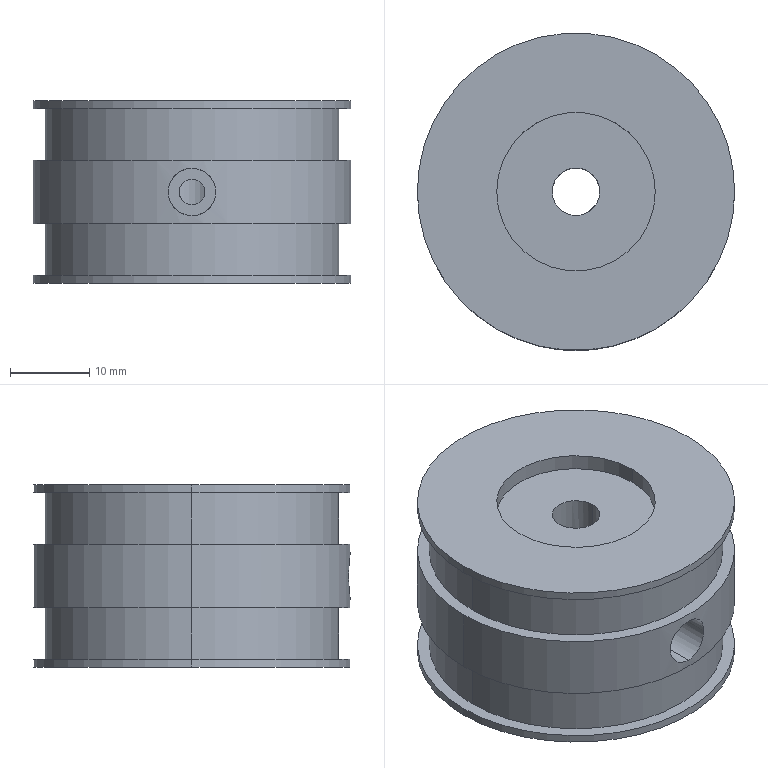Part | SolidWorks | features BaseBody 1 | 1 solid | 32 faces | box 40 x 40 x 23 mm | volume 24363 mm3 | cylinder 22 | plane 10 | commonest cylinder face diameters 40 x6 3.242 x4 6 x4 20 x4 37 x4
STEP:
#1=CARTESIAN_POINT('',(-161.861,-352.289,7.5));
#2=VERTEX_POINT('',#1);
#3=CARTESIAN_POINT('',(-201.861,-352.289,7.5));
#4=VERTEX_POINT('',#3);
#5=CARTESIAN_POINT('',(-181.861,-352.289,7.5));
#6=DIRECTION('',(0.,0.,1.));
#7=DIRECTION('',(1.,0.,0.));
#8=AXIS2_PLACEMENT_3D('',#5,#6,#7);
#9=CIRCLE('',#8,20.);
#10=EDGE_CURVE('',#2,#4,#9,.T.);
#11=ORIENTED_EDGE('',*,*,#10,.T.);
#12=CARTESIAN_POINT('',(-201.861,-352.289,15.5));
#13=VERTEX_POINT('',#12);
#14=CARTESIAN_POINT('',(-201.861,-352.289,0.));
#15=DIRECTION('',(0.,0.,1.));
#16=VECTOR('',#15,1000.);
#17=LINE('',#14,#16);
#18=EDGE_CURVE('',#4,#13,#17,.T.);
#19=ORIENTED_EDGE('',*,*,#18,.T.);
#20=CARTESIAN_POINT('',(-161.861,-352.289,15.5));
#21=VERTEX_POINT('',#20);
#22=CARTESIAN_POINT('',(-181.861,-352.289,15.5));
#23=DIRECTION('',(0.,0.,-1.));
#24=DIRECTION('',(1.,0.,0.));
#25=AXIS2_PLACEMENT_3D('',#22,#23,#24);
#26=CIRCLE('',#25,20.);
#27=EDGE_CURVE('',#13,#21,#26,.T.);
#28=ORIENTED_EDGE('',*,*,#27,.T.);
#29=CARTESIAN_POINT('',(-161.861,-352.289,0.));
#30=DIRECTION('',(0.,0.,1.));
#31=VECTOR('',#30,1000.);
#32=LINE('',#29,#31);
#33=EDGE_CURVE('',#2,#21,#32,.T.);
#34=ORIENTED_EDGE('',*,*,#33,.F.);
#35=EDGE_LOOP('',(#11,#19,#28,#34));
#36=FACE_OUTER_BOUND('',#35,.T.);
#37=CARTESIAN_POINT('',(-181.861,-352.289,0.));
#38=DIRECTION('',(0.,0.,1.));
#39=DIRECTION('',(1.,0.,0.));
#40=AXIS2_PLACEMENT_3D('',#37,#38,#39);
#41=CYLINDRICAL_SURFACE('',#40,20.);
#42=ADVANCED_FACE('',(#36),#41,.T.);
#43=CARTESIAN_POINT('',(-181.861,-372.289,8.5));
#44=VERTEX_POINT('',#43);
#45=CARTESIAN_POINT('',(-181.861,-372.289,14.5));
#46=VERTEX_POINT('',#45);
#47=CARTESIAN_POINT('',(-181.861,-372.289,8.5));
#48=CARTESIAN_POINT('',(-182.06,-372.289,8.5));
#49=CARTESIAN_POINT('',(-182.255,-372.286,8.52));
#50=CARTESIAN_POINT('',(-182.639,-372.275,8.596));
#51=CARTESIAN_POINT('',(-182.829,-372.266,8.654));
#52=CARTESIAN_POINT('',(-183.193,-372.245,8.804));
#53=CARTESIAN_POINT('',(-183.365,-372.233,8.896));
#54=CARTESIAN_POINT('',(-183.691,-372.206,9.114));
#55=CARTESIAN_POINT('',(-183.845,-372.191,9.241));
#56=CARTESIAN_POINT('',(-184.121,-372.161,9.517));
#57=CARTESIAN_POINT('',(-184.245,-372.147,9.668));
#58=CARTESIAN_POINT('',(-184.464,-372.119,9.995));
#59=CARTESIAN_POINT('',(-184.557,-372.107,10.17));
#60=CARTESIAN_POINT('',(-184.707,-372.086,10.53));
#61=CARTESIAN_POINT('',(-184.765,-372.077,10.72));
#62=CARTESIAN_POINT('',(-184.842,-372.066,11.107));
#63=CARTESIAN_POINT('',(-184.861,-372.063,11.302));
#64=CARTESIAN_POINT('',(-184.862,-372.063,11.694));
#65=CARTESIAN_POINT('',(-184.842,-372.066,11.893));
#66=CARTESIAN_POINT('',(-184.766,-372.077,12.278));
#67=CARTESIAN_POINT('',(-184.709,-372.085,12.465));
#68=CARTESIAN_POINT('',(-184.559,-372.106,12.828));
#69=CARTESIAN_POINT('',(-184.465,-372.119,13.004));
#70=CARTESIAN_POINT('',(-184.248,-372.146,13.328));
#71=CARTESIAN_POINT('',(-184.124,-372.161,13.48));
#72=CARTESIAN_POINT('',(-183.844,-372.191,13.76));
#73=CARTESIAN_POINT('',(-183.693,-372.205,13.884));
#74=CARTESIAN_POINT('',(-183.369,-372.233,14.101));
#75=CARTESIAN_POINT('',(-183.193,-372.245,14.195));
#76=CARTESIAN_POINT('',(-182.83,-372.266,14.346));
#77=CARTESIAN_POINT('',(-182.643,-372.275,14.403));
#78=CARTESIAN_POINT('',(-182.259,-372.286,14.48));
#79=CARTESIAN_POINT('',(-182.06,-372.289,14.5));
#80=CARTESIAN_POINT('',(-181.861,-372.289,14.5));
#81=B_SPLINE_CURVE_WITH_KNOTS('',3,(#47,#48,#49,#50,#51,#52,#53,#54,#55,#56,#57,#58,#59,#60,#61,#62,#63,#64,#65,#66,#67,#68,#69,#70,#71,#72,#73,#74,#75,#76,#77,#78,#79,#80),.UNSPECIFIED.,.F.,.F.,(4,2,2,2,2,2,2,2,2,2,2,2,2,2,2,2,4),(0.00939,0.009977,0.01056,0.01115,0.01174,0.01232,0.01291,0.0135,0.01409,0.01467,0.01526,0.01585,0.01643,0.01702,0.01761,0.01819,0.01878),.UNSPECIFIED.);
#82=EDGE_CURVE('',#44,#46,#81,.T.);
#83=ORIENTED_EDGE('',*,*,#82,.F.);
#84=CARTESIAN_POINT('',(-181.861,-363.289,8.5));
#85=VERTEX_POINT('',#84);
#86=CARTESIAN_POINT('',(-181.861,-367.789,8.5));
#87=DIRECTION('',(0.,1.,0.));
#88=VECTOR('',#87,1000.);
#89=LINE('',#86,#88);
#90=EDGE_CURVE('',#44,#85,#89,.T.);
#91=ORIENTED_EDGE('',*,*,#90,.T.);
#92=CARTESIAN_POINT('',(-181.861,-363.289,14.5));
#93=VERTEX_POINT('',#92);
#94=CARTESIAN_POINT('',(-181.861,-363.289,11.5));
#95=DIRECTION('',(0.,-1.,0.));
#96=DIRECTION('',(0.,0.,1.));
#97=AXIS2_PLACEMENT_3D('',#94,#95,#96);
#98=CIRCLE('',#97,3.);
#99=EDGE_CURVE('',#93,#85,#98,.T.);
#100=ORIENTED_EDGE('',*,*,#99,.F.);
#101=CARTESIAN_POINT('',(-181.861,-367.789,14.5));
#102=DIRECTION('',(0.,1.,0.));
#103=VECTOR('',#102,1000.);
#104=LINE('',#101,#103);
#105=EDGE_CURVE('',#46,#93,#104,.T.);
#106=ORIENTED_EDGE('',*,*,#105,.F.);
#107=EDGE_LOOP('',(#83,#91,#100,#106));
#108=FACE_OUTER_BOUND('',#107,.T.);
#109=CARTESIAN_POINT('',(-181.861,-367.789,11.5));
#110=DIRECTION('',(0.,1.,0.));
#111=DIRECTION('',(0.,0.,1.));
#112=AXIS2_PLACEMENT_3D('',#109,#110,#111);
#113=CYLINDRICAL_SURFACE('',#112,3.);
#114=ADVANCED_FACE('',(#108),#113,.F.);
#115=CARTESIAN_POINT('',(-163.361,-352.289,1.));
#116=VERTEX_POINT('',#115);
#117=CARTESIAN_POINT('',(-200.361,-352.289,1.));
#118=VERTEX_POINT('',#117);
#119=CARTESIAN_POINT('',(-181.861,-352.289,1.));
#120=DIRECTION('',(0.,0.,1.));
#121=DIRECTION('',(1.,0.,0.));
#122=AXIS2_PLACEMENT_3D('',#119,#120,#121);
#123=CIRCLE('',#122,18.5);
#124=EDGE_CURVE('',#116,#118,#123,.T.);
#125=ORIENTED_EDGE('',*,*,#124,.T.);
#126=CARTESIAN_POINT('',(-200.361,-352.289,7.5));
#127=VERTEX_POINT('',#126);
#128=CARTESIAN_POINT('',(-200.361,-352.289,4.25));
#129=DIRECTION('',(0.,0.,1.));
#130=VECTOR('',#129,1000.);
#131=LINE('',#128,#130);
#132=EDGE_CURVE('',#118,#127,#131,.T.);
#133=ORIENTED_EDGE('',*,*,#132,.T.);
#134=CARTESIAN_POINT('',(-163.361,-352.289,7.5));
#135=VERTEX_POINT('',#134);
#136=CARTESIAN_POINT('',(-181.861,-352.289,7.5));
#137=DIRECTION('',(0.,0.,-1.));
#138=DIRECTION('',(1.,0.,0.));
#139=AXIS2_PLACEMENT_3D('',#136,#137,#138);
#140=CIRCLE('',#139,18.5);
#141=EDGE_CURVE('',#127,#135,#140,.T.);
#142=ORIENTED_EDGE('',*,*,#141,.T.);
#143=CARTESIAN_POINT('',(-163.361,-352.289,4.25));
#144=DIRECTION('',(0.,0.,1.));
#145=VECTOR('',#144,1000.);
#146=LINE('',#143,#145);
#147=EDGE_CURVE('',#116,#135,#146,.T.);
#148=ORIENTED_EDGE('',*,*,#147,.F.);
#149=EDGE_LOOP('',(#125,#133,#142,#148));
#150=FACE_OUTER_BOUND('',#149,.T.);
#151=CARTESIAN_POINT('',(-181.861,-352.289,4.25));
#152=DIRECTION('',(0.,0.,1.));
#153=DIRECTION('',(1.,0.,0.));
#154=AXIS2_PLACEMENT_3D('',#151,#152,#153);
#155=CYLINDRICAL_SURFACE('',#154,18.5);
#156=ADVANCED_FACE('',(#150),#155,.T.);
#157=CARTESIAN_POINT('',(-163.361,-352.289,15.5));
#158=VERTEX_POINT('',#157);
#159=CARTESIAN_POINT('',(-200.361,-352.289,15.5));
#160=VERTEX_POINT('',#159);
#161=CARTESIAN_POINT('',(-181.861,-352.289,15.5));
#162=DIRECTION('',(0.,0.,1.));
#163=DIRECTION('',(1.,0.,0.));
#164=AXIS2_PLACEMENT_3D('',#161,#162,#163);
#165=CIRCLE('',#164,18.5);
#166=EDGE_CURVE('',#158,#160,#165,.T.);
#167=ORIENTED_EDGE('',*,*,#166,.T.);
#168=CARTESIAN_POINT('',(-200.361,-352.289,22.));
#169=VERTEX_POINT('',#168);
#170=CARTESIAN_POINT('',(-200.361,-352.289,18.75));
#171=DIRECTION('',(0.,0.,1.));
#172=VECTOR('',#171,1000.);
#173=LINE('',#170,#172);
#174=EDGE_CURVE('',#160,#169,#173,.T.);
#175=ORIENTED_EDGE('',*,*,#174,.T.);
#176=CARTESIAN_POINT('',(-163.361,-352.289,22.));
#177=VERTEX_POINT('',#176);
#178=CARTESIAN_POINT('',(-181.861,-352.289,22.));
#179=DIRECTION('',(0.,0.,-1.));
#180=DIRECTION('',(1.,0.,0.));
#181=AXIS2_PLACEMENT_3D('',#178,#179,#180);
#182=CIRCLE('',#181,18.5);
#183=EDGE_CURVE('',#169,#177,#182,.T.);
#184=ORIENTED_EDGE('',*,*,#183,.T.);
#185=CARTESIAN_POINT('',(-163.361,-352.289,18.75));
#186=DIRECTION('',(0.,0.,1.));
#187=VECTOR('',#186,1000.);
#188=LINE('',#185,#187);
#189=EDGE_CURVE('',#158,#177,#188,.T.);
#190=ORIENTED_EDGE('',*,*,#189,.F.);
#191=EDGE_LOOP('',(#167,#175,#184,#190));
#192=FACE_OUTER_BOUND('',#191,.T.);
#193=CARTESIAN_POINT('',(-181.861,-352.289,18.75));
#194=DIRECTION('',(0.,0.,1.));
#195=DIRECTION('',(1.,0.,0.));
#196=AXIS2_PLACEMENT_3D('',#193,#194,#195);
#197=CYLINDRICAL_SURFACE('',#196,18.5);
#198=ADVANCED_FACE('',(#192),#197,.T.);
#199=CARTESIAN_POINT('',(-181.861,-355.289,13.121));
#200=VERTEX_POINT('',#199);
#201=CARTESIAN_POINT('',(-181.861,-355.289,9.879));
#202=VERTEX_POINT('',#201);
#203=CARTESIAN_POINT('',(-181.861,-355.289,13.121));
#204=CARTESIAN_POINT('',(-181.969,-355.289,13.121));
#205=CARTESIAN_POINT('',(-182.079,-355.283,13.11));
#206=CARTESIAN_POINT('',(-182.29,-355.26,13.067));
#207=CARTESIAN_POINT('',(-182.392,-355.243,13.035));
#208=CARTESIAN_POINT('',(-182.689,-355.18,12.91));
#209=CARTESIAN_POINT('',(-182.864,-355.121,12.79));
#210=CARTESIAN_POINT('',(-183.084,-355.029,12.569));
#211=CARTESIAN_POINT('',(-183.15,-354.999,12.489));
#212=CARTESIAN_POINT('',(-183.266,-354.94,12.315));
#213=CARTESIAN_POINT('',(-183.317,-354.913,12.222));
#214=CARTESIAN_POINT('',(-183.398,-354.866,12.028));
#215=CARTESIAN_POINT('',(-183.429,-354.847,11.926));
#216=CARTESIAN_POINT('',(-183.472,-354.82,11.714));
#217=CARTESIAN_POINT('',(-183.483,-354.813,11.605));
#218=CARTESIAN_POINT('',(-183.482,-354.813,11.386));
#219=CARTESIAN_POINT('',(-183.471,-354.821,11.279));
#220=CARTESIAN_POINT('',(-183.428,-354.848,11.069));
#221=CARTESIAN_POINT('',(-183.396,-354.867,10.966));
#222=CARTESIAN_POINT('',(-183.272,-354.938,10.674));
#223=CARTESIAN_POINT('',(-183.153,-355.001,10.499));
#224=CARTESIAN_POINT('',(-182.86,-355.122,10.206));
#225=CARTESIAN_POINT('',(-182.683,-355.181,10.087));
#226=CARTESIAN_POINT('',(-182.391,-355.243,9.964));
#227=CARTESIAN_POINT('',(-182.287,-355.26,9.932));
#228=CARTESIAN_POINT('',(-182.077,-355.283,9.89));
#229=CARTESIAN_POINT('',(-181.97,-355.289,9.879));
#230=CARTESIAN_POINT('',(-181.861,-355.289,9.879));
#231=B_SPLINE_CURVE_WITH_KNOTS('',3,(#203,#204,#205,#206,#207,#208,#209,#210,#211,#212,#213,#214,#215,#216,#217,#218,#219,#220,#221,#222,#223,#224,#225,#226,#227,#228,#229,#230),.UNSPECIFIED.,.F.,.F.,(4,2,2,2,2,2,2,2,2,2,2,2,2,4),(0.007755,0.008078,0.0084,0.009046,0.009369,0.009692,0.01001,0.01034,0.01066,0.01098,0.01163,0.01227,0.0126,0.01292),.UNSPECIFIED.);
#232=EDGE_CURVE('',#200,#202,#231,.T.);
#233=ORIENTED_EDGE('',*,*,#232,.F.);
#234=CARTESIAN_POINT('',(-181.861,-363.289,13.121));
#235=VERTEX_POINT('',#234);
#236=CARTESIAN_POINT('',(-181.861,-302.222,13.121));
#237=DIRECTION('',(0.,-1.,0.));
#238=VECTOR('',#237,1000.);
#239=LINE('',#236,#238);
#240=EDGE_CURVE('',#200,#235,#239,.T.);
#241=ORIENTED_EDGE('',*,*,#240,.T.);
#242=CARTESIAN_POINT('',(-181.861,-363.289,9.879));
#243=VERTEX_POINT('',#242);
#244=CARTESIAN_POINT('',(-181.861,-363.289,11.5));
#245=DIRECTION('',(0.,-1.,0.));
#246=DIRECTION('',(0.,0.,-1.));
#247=AXIS2_PLACEMENT_3D('',#244,#245,#246);
#248=CIRCLE('',#247,1.621);
#249=EDGE_CURVE('',#235,#243,#248,.T.);
#250=ORIENTED_EDGE('',*,*,#249,.T.);
#251=CARTESIAN_POINT('',(-181.861,-302.222,9.879));
#252=DIRECTION('',(0.,-1.,0.));
#253=VECTOR('',#252,1000.);
#254=LINE('',#251,#253);
#255=EDGE_CURVE('',#202,#243,#254,.T.);
#256=ORIENTED_EDGE('',*,*,#255,.F.);
#257=EDGE_LOOP('',(#233,#241,#250,#256));
#258=FACE_OUTER_BOUND('',#257,.T.);
#259=CARTESIAN_POINT('',(-181.861,-302.222,11.5));
#260=DIRECTION('',(0.,-1.,0.));
#261=DIRECTION('',(0.,0.,-1.));
#262=AXIS2_PLACEMENT_3D('',#259,#260,#261);
#263=CYLINDRICAL_SURFACE('',#262,1.621);
#264=ADVANCED_FACE('',(#258),#263,.F.);
#265=CARTESIAN_POINT('',(-181.861,-355.289,9.879));
#266=CARTESIAN_POINT('',(-181.645,-355.289,9.879));
#267=CARTESIAN_POINT('',(-181.428,-355.264,9.923));
#268=CARTESIAN_POINT('',(-181.035,-355.18,10.089));
#269=CARTESIAN_POINT('',(-180.859,-355.121,10.209));
#270=CARTESIAN_POINT('',(-180.567,-355.,10.503));
#271=CARTESIAN_POINT('',(-180.448,-354.937,10.679));
#272=CARTESIAN_POINT('',(-180.326,-354.867,10.97));
#273=CARTESIAN_POINT('',(-180.294,-354.847,11.073));
#274=CARTESIAN_POINT('',(-180.251,-354.82,11.284));
#275=CARTESIAN_POINT('',(-180.241,-354.813,11.391));
#276=CARTESIAN_POINT('',(-180.24,-354.813,11.606));
#277=CARTESIAN_POINT('',(-180.251,-354.82,11.716));
#278=CARTESIAN_POINT('',(-180.294,-354.847,11.927));
#279=CARTESIAN_POINT('',(-180.326,-354.866,12.029));
#280=CARTESIAN_POINT('',(-180.408,-354.914,12.226));
#281=CARTESIAN_POINT('',(-180.458,-354.941,12.318));
#282=CARTESIAN_POINT('',(-180.574,-355.,12.491));
#283=CARTESIAN_POINT('',(-180.642,-355.031,12.572));
#284=CARTESIAN_POINT('',(-180.861,-355.122,12.793));
#285=CARTESIAN_POINT('',(-181.039,-355.181,12.913));
#286=CARTESIAN_POINT('',(-181.428,-355.264,13.076));
#287=CARTESIAN_POINT('',(-181.646,-355.289,13.121));
#288=CARTESIAN_POINT('',(-181.861,-355.289,13.121));
#289=B_SPLINE_CURVE_WITH_KNOTS('',3,(#265,#266,#267,#268,#269,#270,#271,#272,#273,#274,#275,#276,#277,#278,#279,#280,#281,#282,#283,#284,#285,#286,#287,#288),.UNSPECIFIED.,.F.,.F.,(4,2,2,2,2,2,2,2,2,2,2,4),(0.002587,0.003233,0.003879,0.004525,0.004848,0.005171,0.005494,0.005817,0.00614,0.006463,0.007109,0.007755),.UNSPECIFIED.);
#290=EDGE_CURVE('',#202,#200,#289,.T.);
#291=ORIENTED_EDGE('',*,*,#290,.T.);
#292=ORIENTED_EDGE('',*,*,#232,.T.);
#293=EDGE_LOOP('',(#291,#292));
#294=FACE_BOUND('',#293,.T.);
#295=CARTESIAN_POINT('',(-178.861,-352.289,21.));
#296=VERTEX_POINT('',#295);
#297=CARTESIAN_POINT('',(-184.861,-352.289,21.));
#298=VERTEX_POINT('',#297);
#299=CARTESIAN_POINT('',(-181.861,-352.289,21.));
#300=DIRECTION('',(0.,0.,-1.));
#301=DIRECTION('',(-1.,0.,0.));
#302=AXIS2_PLACEMENT_3D('',#299,#300,#301);
#303=CIRCLE('',#302,3.);
#304=EDGE_CURVE('',#296,#298,#303,.T.);
#305=ORIENTED_EDGE('',*,*,#304,.F.);
#306=CARTESIAN_POINT('',(-178.861,-352.289,13.121));
#307=VERTEX_POINT('',#306);
#308=CARTESIAN_POINT('',(-178.861,-352.289,63.066));
#309=DIRECTION('',(0.,0.,-1.));
#310=VECTOR('',#309,1000.);
#311=LINE('',#308,#310);
#312=EDGE_CURVE('',#296,#307,#311,.T.);
#313=ORIENTED_EDGE('',*,*,#312,.T.);
#314=CARTESIAN_POINT('',(-179.337,-353.91,11.5));
#315=VERTEX_POINT('',#314);
#316=CARTESIAN_POINT('',(-179.337,-353.91,11.5));
#317=CARTESIAN_POINT('',(-179.337,-353.91,11.61));
#318=CARTESIAN_POINT('',(-179.33,-353.899,11.717));
#319=CARTESIAN_POINT('',(-179.303,-353.856,11.927));
#320=CARTESIAN_POINT('',(-179.284,-353.824,12.031));
#321=CARTESIAN_POINT('',(-179.213,-353.701,12.323));
#322=CARTESIAN_POINT('',(-179.15,-353.582,12.499));
#323=CARTESIAN_POINT('',(-179.029,-353.289,12.792));
#324=CARTESIAN_POINT('',(-178.97,-353.112,12.912));
#325=CARTESIAN_POINT('',(-178.907,-352.82,13.035));
#326=CARTESIAN_POINT('',(-178.89,-352.715,13.068));
#327=CARTESIAN_POINT('',(-178.867,-352.504,13.11));
#328=CARTESIAN_POINT('',(-178.861,-352.397,13.121));
#329=CARTESIAN_POINT('',(-178.861,-352.289,13.121));
#330=B_SPLINE_CURVE_WITH_KNOTS('',3,(#316,#317,#318,#319,#320,#321,#322,#323,#324,#325,#326,#327,#328,#329),.UNSPECIFIED.,.F.,.F.,(4,2,2,2,2,2,4),(0.,0.0003234,0.0006469,0.001294,0.001941,0.002264,0.002587),.UNSPECIFIED.);
#331=EDGE_CURVE('',#315,#307,#330,.T.);
#332=ORIENTED_EDGE('',*,*,#331,.F.);
#333=CARTESIAN_POINT('',(-178.861,-352.289,9.879));
#334=VERTEX_POINT('',#333);
#335=CARTESIAN_POINT('',(-178.861,-352.289,9.879));
#336=CARTESIAN_POINT('',(-178.861,-352.397,9.879));
#337=CARTESIAN_POINT('',(-178.867,-352.506,9.89));
#338=CARTESIAN_POINT('',(-178.89,-352.717,9.933));
#339=CARTESIAN_POINT('',(-178.907,-352.819,9.964));
#340=CARTESIAN_POINT('',(-178.97,-353.115,10.089));
#341=CARTESIAN_POINT('',(-179.029,-353.29,10.209));
#342=CARTESIAN_POINT('',(-179.12,-353.51,10.429));
#343=CARTESIAN_POINT('',(-179.151,-353.576,10.509));
#344=CARTESIAN_POINT('',(-179.209,-353.692,10.682));
#345=CARTESIAN_POINT('',(-179.237,-353.743,10.776));
#346=CARTESIAN_POINT('',(-179.284,-353.824,10.969));
#347=CARTESIAN_POINT('',(-179.303,-353.856,11.07));
#348=CARTESIAN_POINT('',(-179.33,-353.899,11.282));
#349=CARTESIAN_POINT('',(-179.337,-353.91,11.391));
#350=CARTESIAN_POINT('',(-179.337,-353.91,11.5));
#351=B_SPLINE_CURVE_WITH_KNOTS('',3,(#335,#336,#337,#338,#339,#340,#341,#342,#343,#344,#345,#346,#347,#348,#349,#350),.UNSPECIFIED.,.F.,.F.,(4,2,2,2,2,2,2,4),(0.007755,0.008077,0.008399,0.009044,0.009366,0.009688,0.01001,0.01033),.UNSPECIFIED.);
#352=EDGE_CURVE('',#334,#315,#351,.T.);
#353=ORIENTED_EDGE('',*,*,#352,.F.);
#354=CARTESIAN_POINT('',(-178.861,-352.289,2.));
#355=VERTEX_POINT('',#354);
#356=CARTESIAN_POINT('',(-178.861,-352.289,63.066));
#357=DIRECTION('',(0.,0.,-1.));
#358=VECTOR('',#357,1000.);
#359=LINE('',#356,#358);
#360=EDGE_CURVE('',#334,#355,#359,.T.);
#361=ORIENTED_EDGE('',*,*,#360,.T.);
#362=CARTESIAN_POINT('',(-184.861,-352.289,2.));
#363=VERTEX_POINT('',#362);
#364=CARTESIAN_POINT('',(-181.861,-352.289,2.));
#365=DIRECTION('',(0.,0.,1.));
#366=DIRECTION('',(-1.,0.,0.));
#367=AXIS2_PLACEMENT_3D('',#364,#365,#366);
#368=CIRCLE('',#367,3.);
#369=EDGE_CURVE('',#363,#355,#368,.T.);
#370=ORIENTED_EDGE('',*,*,#369,.F.);
#371=CARTESIAN_POINT('',(-184.861,-352.289,63.066));
#372=DIRECTION('',(0.,0.,-1.));
#373=VECTOR('',#372,1000.);
#374=LINE('',#371,#373);
#375=EDGE_CURVE('',#298,#363,#374,.T.);
#376=ORIENTED_EDGE('',*,*,#375,.F.);
#377=EDGE_LOOP('',(#305,#313,#332,#353,#361,#370,#376));
#378=FACE_OUTER_BOUND('',#377,.T.);
#379=CARTESIAN_POINT('',(-181.861,-352.289,63.066));
#380=DIRECTION('',(0.,0.,-1.));
#381=DIRECTION('',(-1.,0.,0.));
#382=AXIS2_PLACEMENT_3D('',#379,#380,#381);
#383=CYLINDRICAL_SURFACE('',#382,3.);
#384=ADVANCED_FACE('',(#294,#378),#383,.F.);
#385=CARTESIAN_POINT('',(-161.861,-352.289,0.));
#386=VERTEX_POINT('',#385);
#387=CARTESIAN_POINT('',(-201.861,-352.289,0.));
#388=VERTEX_POINT('',#387);
#389=CARTESIAN_POINT('',(-181.861,-352.289,0.));
#390=DIRECTION('',(0.,0.,1.));
#391=DIRECTION('',(1.,0.,0.));
#392=AXIS2_PLACEMENT_3D('',#389,#390,#391);
#393=CIRCLE('',#392,20.);
#394=EDGE_CURVE('',#386,#388,#393,.T.);
#395=ORIENTED_EDGE('',*,*,#394,.T.);
#396=CARTESIAN_POINT('',(-201.861,-352.289,1.));
#397=VERTEX_POINT('',#396);
#398=CARTESIAN_POINT('',(-201.861,-352.289,0.));
#399=DIRECTION('',(0.,0.,1.));
#400=VECTOR('',#399,1000.);
#401=LINE('',#398,#400);
#402=EDGE_CURVE('',#388,#397,#401,.T.);
#403=ORIENTED_EDGE('',*,*,#402,.T.);
#404=CARTESIAN_POINT('',(-161.861,-352.289,1.));
#405=VERTEX_POINT('',#404);
#406=CARTESIAN_POINT('',(-181.861,-352.289,1.));
#407=DIRECTION('',(0.,0.,-1.));
#408=DIRECTION('',(1.,0.,0.));
#409=AXIS2_PLACEMENT_3D('',#406,#407,#408);
#410=CIRCLE('',#409,20.);
#411=EDGE_CURVE('',#397,#405,#410,.T.);
#412=ORIENTED_EDGE('',*,*,#411,.T.);
#413=CARTESIAN_POINT('',(-161.861,-352.289,0.));
#414=DIRECTION('',(0.,0.,1.));
#415=VECTOR('',#414,1000.);
#416=LINE('',#413,#415);
#417=EDGE_CURVE('',#386,#405,#416,.T.);
#418=ORIENTED_EDGE('',*,*,#417,.F.);
#419=EDGE_LOOP('',(#395,#403,#412,#418));
#420=FACE_OUTER_BOUND('',#419,.T.);
#421=CARTESIAN_POINT('',(-181.861,-352.289,0.));
#422=DIRECTION('',(0.,0.,1.));
#423=DIRECTION('',(1.,0.,0.));
#424=AXIS2_PLACEMENT_3D('',#421,#422,#423);
#425=CYLINDRICAL_SURFACE('',#424,20.);
#426=ADVANCED_FACE('',(#420),#425,.T.);
#427=CARTESIAN_POINT('',(-161.861,-352.289,22.));
#428=VERTEX_POINT('',#427);
#429=CARTESIAN_POINT('',(-201.861,-352.289,22.));
#430=VERTEX_POINT('',#429);
#431=CARTESIAN_POINT('',(-181.861,-352.289,22.));
#432=DIRECTION('',(0.,0.,1.));
#433=DIRECTION('',(1.,0.,0.));
#434=AXIS2_PLACEMENT_3D('',#431,#432,#433);
#435=CIRCLE('',#434,20.);
#436=EDGE_CURVE('',#428,#430,#435,.T.);
#437=ORIENTED_EDGE('',*,*,#436,.T.);
#438=CARTESIAN_POINT('',(-201.861,-352.289,23.));
#439=VERTEX_POINT('',#438);
#440=CARTESIAN_POINT('',(-201.861,-352.289,0.));
#441=DIRECTION('',(0.,0.,1.));
#442=VECTOR('',#441,1000.);
#443=LINE('',#440,#442);
#444=EDGE_CURVE('',#430,#439,#443,.T.);
#445=ORIENTED_EDGE('',*,*,#444,.T.);
#446=CARTESIAN_POINT('',(-161.861,-352.289,23.));
#447=VERTEX_POINT('',#446);
#448=CARTESIAN_POINT('',(-181.861,-352.289,23.));
#449=DIRECTION('',(0.,0.,-1.));
#450=DIRECTION('',(1.,0.,0.));
#451=AXIS2_PLACEMENT_3D('',#448,#449,#450);
#452=CIRCLE('',#451,20.);
#453=EDGE_CURVE('',#439,#447,#452,.T.);
#454=ORIENTED_EDGE('',*,*,#453,.T.);
#455=CARTESIAN_POINT('',(-161.861,-352.289,0.));
#456=DIRECTION('',(0.,0.,1.));
#457=VECTOR('',#456,1000.);
#458=LINE('',#455,#457);
#459=EDGE_CURVE('',#428,#447,#458,.T.);
#460=ORIENTED_EDGE('',*,*,#459,.F.);
#461=EDGE_LOOP('',(#437,#445,#454,#460));
#462=FACE_OUTER_BOUND('',#461,.T.);
#463=CARTESIAN_POINT('',(-181.861,-352.289,0.));
#464=DIRECTION('',(0.,0.,1.));
#465=DIRECTION('',(1.,0.,0.));
#466=AXIS2_PLACEMENT_3D('',#463,#464,#465);
#467=CYLINDRICAL_SURFACE('',#466,20.);
#468=ADVANCED_FACE('',(#462),#467,.T.);
#469=CARTESIAN_POINT('',(-179.337,-350.668,11.5));
#470=VERTEX_POINT('',#469);
#471=CARTESIAN_POINT('',(-179.337,-350.668,11.5));
#472=CARTESIAN_POINT('',(-179.337,-350.668,11.392));
#473=CARTESIAN_POINT('',(-179.33,-350.679,11.282));
#474=CARTESIAN_POINT('',(-179.303,-350.722,11.072));
#475=CARTESIAN_POINT('',(-179.284,-350.753,10.97));
#476=CARTESIAN_POINT('',(-179.236,-350.836,10.773));
#477=CARTESIAN_POINT('',(-179.209,-350.886,10.681));
#478=CARTESIAN_POINT('',(-179.15,-351.002,10.508));
#479=CARTESIAN_POINT('',(-179.119,-351.07,10.427));
#480=CARTESIAN_POINT('',(-179.028,-351.289,10.207));
#481=CARTESIAN_POINT('',(-178.969,-351.467,10.087));
#482=CARTESIAN_POINT('',(-178.886,-351.856,9.924));
#483=CARTESIAN_POINT('',(-178.861,-352.073,9.879));
#484=CARTESIAN_POINT('',(-178.861,-352.289,9.879));
#485=B_SPLINE_CURVE_WITH_KNOTS('',3,(#471,#472,#473,#474,#475,#476,#477,#478,#479,#480,#481,#482,#483,#484),.UNSPECIFIED.,.F.,.F.,(4,2,2,2,2,2,4),(0.005173,0.005495,0.005818,0.006141,0.006464,0.007109,0.007755),.UNSPECIFIED.);
#486=EDGE_CURVE('',#470,#334,#485,.T.);
#487=ORIENTED_EDGE('',*,*,#486,.T.);
#488=ORIENTED_EDGE('',*,*,#352,.T.);
#489=CARTESIAN_POINT('',(-170.861,-353.91,11.5));
#490=VERTEX_POINT('',#489);
#491=CARTESIAN_POINT('',(-231.928,-353.91,11.5));
#492=DIRECTION('',(1.,0.,0.));
#493=VECTOR('',#492,1000.);
#494=LINE('',#491,#493);
#495=EDGE_CURVE('',#315,#490,#494,.T.);
#496=ORIENTED_EDGE('',*,*,#495,.T.);
#497=CARTESIAN_POINT('',(-170.861,-350.668,11.5));
#498=VERTEX_POINT('',#497);
#499=CARTESIAN_POINT('',(-170.861,-352.289,11.5));
#500=DIRECTION('',(-1.,0.,0.));
#501=DIRECTION('',(0.,1.,0.));
#502=AXIS2_PLACEMENT_3D('',#499,#500,#501);
#503=CIRCLE('',#502,1.621);
#504=EDGE_CURVE('',#498,#490,#503,.T.);
#505=ORIENTED_EDGE('',*,*,#504,.F.);
#506=CARTESIAN_POINT('',(-231.928,-350.668,11.5));
#507=DIRECTION('',(1.,0.,0.));
#508=VECTOR('',#507,1000.);
#509=LINE('',#506,#508);
#510=EDGE_CURVE('',#470,#498,#509,.T.);
#511=ORIENTED_EDGE('',*,*,#510,.F.);
#512=EDGE_LOOP('',(#487,#488,#496,#505,#511));
#513=FACE_OUTER_BOUND('',#512,.T.);
#514=CARTESIAN_POINT('',(-231.928,-352.289,11.5));
#515=DIRECTION('',(1.,0.,0.));
#516=DIRECTION('',(0.,1.,0.));
#517=AXIS2_PLACEMENT_3D('',#514,#515,#516);
#518=CYLINDRICAL_SURFACE('',#517,1.621);
#519=ADVANCED_FACE('',(#513),#518,.F.);
#520=CARTESIAN_POINT('',(-191.861,-352.289,0.));
#521=VERTEX_POINT('',#520);
#522=CARTESIAN_POINT('',(-171.861,-352.289,0.));
#523=VERTEX_POINT('',#522);
#524=CARTESIAN_POINT('',(-181.861,-352.289,0.));
#525=DIRECTION('',(0.,0.,1.));
#526=DIRECTION('',(1.,0.,0.));
#527=AXIS2_PLACEMENT_3D('',#524,#525,#526);
#528=CIRCLE('',#527,10.);
#529=EDGE_CURVE('',#521,#523,#528,.T.);
#530=ORIENTED_EDGE('',*,*,#529,.F.);
#531=CARTESIAN_POINT('',(-191.861,-352.289,2.));
#532=VERTEX_POINT('',#531);
#533=CARTESIAN_POINT('',(-191.861,-352.289,0.));
#534=DIRECTION('',(0.,0.,1.));
#535=VECTOR('',#534,1000.);
#536=LINE('',#533,#535);
#537=EDGE_CURVE('',#521,#532,#536,.T.);
#538=ORIENTED_EDGE('',*,*,#537,.T.);
#539=CARTESIAN_POINT('',(-171.861,-352.289,2.));
#540=VERTEX_POINT('',#539);
#541=CARTESIAN_POINT('',(-181.861,-352.289,2.));
#542=DIRECTION('',(0.,0.,1.));
#543=DIRECTION('',(1.,0.,0.));
#544=AXIS2_PLACEMENT_3D('',#541,#542,#543);
#545=CIRCLE('',#544,10.);
#546=EDGE_CURVE('',#532,#540,#545,.T.);
#547=ORIENTED_EDGE('',*,*,#546,.T.);
#548=CARTESIAN_POINT('',(-171.861,-352.289,0.));
#549=DIRECTION('',(0.,0.,1.));
#550=VECTOR('',#549,1000.);
#551=LINE('',#548,#550);
#552=EDGE_CURVE('',#523,#540,#551,.T.);
#553=ORIENTED_EDGE('',*,*,#552,.F.);
#554=EDGE_LOOP('',(#530,#538,#547,#553));
#555=FACE_OUTER_BOUND('',#554,.T.);
#556=CARTESIAN_POINT('',(-181.861,-352.289,0.));
#557=DIRECTION('',(0.,0.,1.));
#558=DIRECTION('',(1.,0.,0.));
#559=AXIS2_PLACEMENT_3D('',#556,#557,#558);
#560=CYLINDRICAL_SURFACE('',#559,10.);
#561=ADVANCED_FACE('',(#555),#560,.F.);
#562=CARTESIAN_POINT('',(-191.861,-352.289,23.));
#563=VERTEX_POINT('',#562);
#564=CARTESIAN_POINT('',(-171.861,-352.289,23.));
#565=VERTEX_POINT('',#564);
#566=CARTESIAN_POINT('',(-181.861,-352.289,23.));
#567=DIRECTION('',(0.,0.,1.));
#568=DIRECTION('',(-1.,0.,0.));
#569=AXIS2_PLACEMENT_3D('',#566,#567,#568);
#570=CIRCLE('',#569,10.);
#571=EDGE_CURVE('',#563,#565,#570,.T.);
#572=ORIENTED_EDGE('',*,*,#571,.T.);
#573=CARTESIAN_POINT('',(-171.861,-352.289,21.));
#574=VERTEX_POINT('',#573);
#575=CARTESIAN_POINT('',(-171.861,-352.289,23.));
#576=DIRECTION('',(0.,0.,-1.));
#577=VECTOR('',#576,1000.);
#578=LINE('',#575,#577);
#579=EDGE_CURVE('',#565,#574,#578,.T.);
#580=ORIENTED_EDGE('',*,*,#579,.T.);
#581=CARTESIAN_POINT('',(-191.861,-352.289,21.));
#582=VERTEX_POINT('',#581);
#583=CARTESIAN_POINT('',(-181.861,-352.289,21.));
#584=DIRECTION('',(0.,0.,-1.));
#585=DIRECTION('',(-1.,0.,0.));
#586=AXIS2_PLACEMENT_3D('',#583,#584,#585);
#587=CIRCLE('',#586,10.);
#588=EDGE_CURVE('',#574,#582,#587,.T.);
#589=ORIENTED_EDGE('',*,*,#588,.T.);
#590=CARTESIAN_POINT('',(-191.861,-352.289,23.));
#591=DIRECTION('',(0.,0.,-1.));
#592=VECTOR('',#591,1000.);
#593=LINE('',#590,#592);
#594=EDGE_CURVE('',#563,#582,#593,.T.);
#595=ORIENTED_EDGE('',*,*,#594,.F.);
#596=EDGE_LOOP('',(#572,#580,#589,#595));
#597=FACE_OUTER_BOUND('',#596,.T.);
#598=CARTESIAN_POINT('',(-181.861,-352.289,23.));
#599=DIRECTION('',(0.,0.,-1.));
#600=DIRECTION('',(-1.,0.,0.));
#601=AXIS2_PLACEMENT_3D('',#598,#599,#600);
#602=CYLINDRICAL_SURFACE('',#601,10.);
#603=ADVANCED_FACE('',(#597),#602,.F.);
#604=ORIENTED_EDGE('',*,*,#18,.F.);
#605=CARTESIAN_POINT('',(-181.861,-352.289,7.5));
#606=DIRECTION('',(0.,0.,1.));
#607=DIRECTION('',(1.,0.,0.));
#608=AXIS2_PLACEMENT_3D('',#605,#606,#607);
#609=CIRCLE('',#608,20.);
#610=EDGE_CURVE('',#4,#2,#609,.T.);
#611=ORIENTED_EDGE('',*,*,#610,.T.);
#612=ORIENTED_EDGE('',*,*,#33,.T.);
#613=CARTESIAN_POINT('',(-181.861,-352.289,15.5));
#614=DIRECTION('',(0.,0.,-1.));
#615=DIRECTION('',(1.,0.,0.));
#616=AXIS2_PLACEMENT_3D('',#613,#614,#615);
#617=CIRCLE('',#616,20.);
#618=EDGE_CURVE('',#21,#13,#617,.T.);
#619=ORIENTED_EDGE('',*,*,#618,.T.);
#620=EDGE_LOOP('',(#604,#611,#612,#619));
#621=FACE_OUTER_BOUND('',#620,.T.);
#622=CARTESIAN_POINT('',(-181.861,-372.289,14.5));
#623=CARTESIAN_POINT('',(-181.663,-372.289,14.5));
#624=CARTESIAN_POINT('',(-181.468,-372.286,14.48));
#625=CARTESIAN_POINT('',(-181.084,-372.275,14.404));
#626=CARTESIAN_POINT('',(-180.893,-372.266,14.346));
#627=CARTESIAN_POINT('',(-180.53,-372.245,14.196));
#628=CARTESIAN_POINT('',(-180.358,-372.233,14.104));
#629=CARTESIAN_POINT('',(-180.032,-372.206,13.886));
#630=CARTESIAN_POINT('',(-179.878,-372.191,13.759));
#631=CARTESIAN_POINT('',(-179.602,-372.161,13.483));
#632=CARTESIAN_POINT('',(-179.478,-372.147,13.332));
#633=CARTESIAN_POINT('',(-179.259,-372.119,13.005));
#634=CARTESIAN_POINT('',(-179.165,-372.107,12.83));
#635=CARTESIAN_POINT('',(-179.016,-372.086,12.47));
#636=CARTESIAN_POINT('',(-178.958,-372.077,12.28));
#637=CARTESIAN_POINT('',(-178.881,-372.066,11.893));
#638=CARTESIAN_POINT('',(-178.862,-372.063,11.698));
#639=CARTESIAN_POINT('',(-178.861,-372.063,11.306));
#640=CARTESIAN_POINT('',(-178.881,-372.066,11.107));
#641=CARTESIAN_POINT('',(-178.957,-372.077,10.722));
#642=CARTESIAN_POINT('',(-179.014,-372.085,10.535));
#643=CARTESIAN_POINT('',(-179.164,-372.106,10.172));
#644=CARTESIAN_POINT('',(-179.258,-372.119,9.996));
#645=CARTESIAN_POINT('',(-179.475,-372.146,9.672));
#646=CARTESIAN_POINT('',(-179.599,-372.161,9.52));
#647=CARTESIAN_POINT('',(-179.879,-372.191,9.24));
#648=CARTESIAN_POINT('',(-180.03,-372.205,9.116));
#649=CARTESIAN_POINT('',(-180.354,-372.233,8.899));
#650=CARTESIAN_POINT('',(-180.53,-372.245,8.805));
#651=CARTESIAN_POINT('',(-180.892,-372.266,8.654));
#652=CARTESIAN_POINT('',(-181.079,-372.275,8.597));
#653=CARTESIAN_POINT('',(-181.464,-372.286,8.52));
#654=CARTESIAN_POINT('',(-181.663,-372.289,8.5));
#655=CARTESIAN_POINT('',(-181.861,-372.289,8.5));
#656=B_SPLINE_CURVE_WITH_KNOTS('',3,(#622,#623,#624,#625,#626,#627,#628,#629,#630,#631,#632,#633,#634,#635,#636,#637,#638,#639,#640,#641,#642,#643,#644,#645,#646,#647,#648,#649,#650,#651,#652,#653,#654,#655),.UNSPECIFIED.,.F.,.F.,(4,2,2,2,2,2,2,2,2,2,2,2,2,2,2,2,4),(0.,0.0005869,0.001174,0.001761,0.002348,0.002934,0.003521,0.004108,0.004695,0.005282,0.005869,0.006456,0.007043,0.00763,0.008217,0.008803,0.00939),.UNSPECIFIED.);
#657=EDGE_CURVE('',#46,#44,#656,.T.);
#658=ORIENTED_EDGE('',*,*,#657,.T.);
#659=ORIENTED_EDGE('',*,*,#82,.T.);
#660=EDGE_LOOP('',(#658,#659));
#661=FACE_BOUND('',#660,.T.);
#662=CARTESIAN_POINT('',(-181.861,-352.289,0.));
#663=DIRECTION('',(0.,0.,1.));
#664=DIRECTION('',(1.,0.,0.));
#665=AXIS2_PLACEMENT_3D('',#662,#663,#664);
#666=CYLINDRICAL_SURFACE('',#665,20.);
#667=ADVANCED_FACE('',(#621,#661),#666,.T.);
#668=ORIENTED_EDGE('',*,*,#90,.F.);
#669=ORIENTED_EDGE('',*,*,#657,.F.);
#670=ORIENTED_EDGE('',*,*,#105,.T.);
#671=CARTESIAN_POINT('',(-181.861,-363.289,11.5));
#672=DIRECTION('',(0.,-1.,0.));
#673=DIRECTION('',(0.,0.,1.));
#674=AXIS2_PLACEMENT_3D('',#671,#672,#673);
#675=CIRCLE('',#674,3.);
#676=EDGE_CURVE('',#85,#93,#675,.T.);
#677=ORIENTED_EDGE('',*,*,#676,.F.);
#678=EDGE_LOOP('',(#668,#669,#670,#677));
#679=FACE_OUTER_BOUND('',#678,.T.);
#680=CARTESIAN_POINT('',(-181.861,-367.789,11.5));
#681=DIRECTION('',(0.,1.,0.));
#682=DIRECTION('',(0.,0.,1.));
#683=AXIS2_PLACEMENT_3D('',#680,#681,#682);
#684=CYLINDRICAL_SURFACE('',#683,3.);
#685=ADVANCED_FACE('',(#679),#684,.F.);
#686=CARTESIAN_POINT('',(-181.861,-352.289,7.5));
#687=DIRECTION('',(0.,0.,-1.));
#688=DIRECTION('',(1.,0.,0.));
#689=AXIS2_PLACEMENT_3D('',#686,#687,#688);
#690=CIRCLE('',#689,18.5);
#691=EDGE_CURVE('',#135,#127,#690,.T.);
#692=ORIENTED_EDGE('',*,*,#691,.F.);
#693=ORIENTED_EDGE('',*,*,#141,.F.);
#694=EDGE_LOOP('',(#692,#693));
#695=FACE_BOUND('',#694,.T.);
#696=ORIENTED_EDGE('',*,*,#10,.F.);
#697=ORIENTED_EDGE('',*,*,#610,.F.);
#698=EDGE_LOOP('',(#696,#697));
#699=FACE_OUTER_BOUND('',#698,.T.);
#700=CARTESIAN_POINT('',(-201.111,-352.289,7.5));
#701=DIRECTION('',(0.,0.,1.));
#702=DIRECTION('',(1.,0.,0.));
#703=AXIS2_PLACEMENT_3D('',#700,#701,#702);
#704=PLANE('',#703);
#705=ADVANCED_FACE('',(#695,#699),#704,.F.);
#706=ORIENTED_EDGE('',*,*,#166,.F.);
#707=CARTESIAN_POINT('',(-181.861,-352.289,15.5));
#708=DIRECTION('',(0.,0.,1.));
#709=DIRECTION('',(1.,0.,0.));
#710=AXIS2_PLACEMENT_3D('',#707,#708,#709);
#711=CIRCLE('',#710,18.5);
#712=EDGE_CURVE('',#160,#158,#711,.T.);
#713=ORIENTED_EDGE('',*,*,#712,.F.);
#714=EDGE_LOOP('',(#706,#713));
#715=FACE_BOUND('',#714,.T.);
#716=ORIENTED_EDGE('',*,*,#618,.F.);
#717=ORIENTED_EDGE('',*,*,#27,.F.);
#718=EDGE_LOOP('',(#716,#717));
#719=FACE_OUTER_BOUND('',#718,.T.);
#720=CARTESIAN_POINT('',(-201.111,-352.289,15.5));
#721=DIRECTION('',(0.,0.,-1.));
#722=DIRECTION('',(-1.,0.,0.));
#723=AXIS2_PLACEMENT_3D('',#720,#721,#722);
#724=PLANE('',#723);
#725=ADVANCED_FACE('',(#715,#719),#724,.F.);
#726=CARTESIAN_POINT('',(-181.861,-363.289,11.5));
#727=DIRECTION('',(0.,-1.,0.));
#728=DIRECTION('',(0.,0.,-1.));
#729=AXIS2_PLACEMENT_3D('',#726,#727,#728);
#730=CIRCLE('',#729,1.621);
#731=EDGE_CURVE('',#243,#235,#730,.T.);
#732=ORIENTED_EDGE('',*,*,#731,.F.);
#733=ORIENTED_EDGE('',*,*,#249,.F.);
#734=EDGE_LOOP('',(#732,#733));
#735=FACE_BOUND('',#734,.T.);
#736=ORIENTED_EDGE('',*,*,#99,.T.);
#737=ORIENTED_EDGE('',*,*,#676,.T.);
#738=EDGE_LOOP('',(#736,#737));
#739=FACE_OUTER_BOUND('',#738,.T.);
#740=CARTESIAN_POINT('',(-181.861,-363.289,11.5));
#741=DIRECTION('',(0.,1.,0.));
#742=DIRECTION('',(0.,0.,1.));
#743=AXIS2_PLACEMENT_3D('',#740,#741,#742);
#744=PLANE('',#743);
#745=ADVANCED_FACE('',(#735,#739),#744,.F.);
#746=ORIENTED_EDGE('',*,*,#132,.F.);
#747=CARTESIAN_POINT('',(-181.861,-352.289,1.));
#748=DIRECTION('',(0.,0.,1.));
#749=DIRECTION('',(1.,0.,0.));
#750=AXIS2_PLACEMENT_3D('',#747,#748,#749);
#751=CIRCLE('',#750,18.5);
#752=EDGE_CURVE('',#118,#116,#751,.T.);
#753=ORIENTED_EDGE('',*,*,#752,.T.);
#754=ORIENTED_EDGE('',*,*,#147,.T.);
#755=ORIENTED_EDGE('',*,*,#691,.T.);
#756=EDGE_LOOP('',(#746,#753,#754,#755));
#757=FACE_OUTER_BOUND('',#756,.T.);
#758=CARTESIAN_POINT('',(-181.861,-352.289,4.25));
#759=DIRECTION('',(0.,0.,1.));
#760=DIRECTION('',(1.,0.,0.));
#761=AXIS2_PLACEMENT_3D('',#758,#759,#760);
#762=CYLINDRICAL_SURFACE('',#761,18.5);
#763=ADVANCED_FACE('',(#757),#762,.T.);
#764=ORIENTED_EDGE('',*,*,#174,.F.);
#765=ORIENTED_EDGE('',*,*,#712,.T.);
#766=ORIENTED_EDGE('',*,*,#189,.T.);
#767=CARTESIAN_POINT('',(-181.861,-352.289,22.));
#768=DIRECTION('',(0.,0.,-1.));
#769=DIRECTION('',(1.,0.,0.));
#770=AXIS2_PLACEMENT_3D('',#767,#768,#769);
#771=CIRCLE('',#770,18.5);
#772=EDGE_CURVE('',#177,#169,#771,.T.);
#773=ORIENTED_EDGE('',*,*,#772,.T.);
#774=EDGE_LOOP('',(#764,#765,#766,#773));
#775=FACE_OUTER_BOUND('',#774,.T.);
#776=CARTESIAN_POINT('',(-181.861,-352.289,18.75));
#777=DIRECTION('',(0.,0.,1.));
#778=DIRECTION('',(1.,0.,0.));
#779=AXIS2_PLACEMENT_3D('',#776,#777,#778);
#780=CYLINDRICAL_SURFACE('',#779,18.5);
#781=ADVANCED_FACE('',(#775),#780,.T.);
#782=ORIENTED_EDGE('',*,*,#240,.F.);
#783=ORIENTED_EDGE('',*,*,#290,.F.);
#784=ORIENTED_EDGE('',*,*,#255,.T.);
#785=ORIENTED_EDGE('',*,*,#731,.T.);
#786=EDGE_LOOP('',(#782,#783,#784,#785));
#787=FACE_OUTER_BOUND('',#786,.T.);
#788=CARTESIAN_POINT('',(-181.861,-302.222,11.5));
#789=DIRECTION('',(0.,-1.,0.));
#790=DIRECTION('',(0.,0.,-1.));
#791=AXIS2_PLACEMENT_3D('',#788,#789,#790);
#792=CYLINDRICAL_SURFACE('',#791,1.621);
#793=ADVANCED_FACE('',(#787),#792,.F.);
#794=ORIENTED_EDGE('',*,*,#124,.F.);
#795=ORIENTED_EDGE('',*,*,#752,.F.);
#796=EDGE_LOOP('',(#794,#795));
#797=FACE_BOUND('',#796,.T.);
#798=CARTESIAN_POINT('',(-181.861,-352.289,1.));
#799=DIRECTION('',(0.,0.,-1.));
#800=DIRECTION('',(1.,0.,0.));
#801=AXIS2_PLACEMENT_3D('',#798,#799,#800);
#802=CIRCLE('',#801,20.);
#803=EDGE_CURVE('',#405,#397,#802,.T.);
#804=ORIENTED_EDGE('',*,*,#803,.F.);
#805=ORIENTED_EDGE('',*,*,#411,.F.);
#806=EDGE_LOOP('',(#804,#805));
#807=FACE_OUTER_BOUND('',#806,.T.);
#808=CARTESIAN_POINT('',(-201.111,-352.289,1.));
#809=DIRECTION('',(0.,0.,-1.));
#810=DIRECTION('',(-1.,0.,0.));
#811=AXIS2_PLACEMENT_3D('',#808,#809,#810);
#812=PLANE('',#811);
#813=ADVANCED_FACE('',(#797,#807),#812,.F.);
#814=ORIENTED_EDGE('',*,*,#772,.F.);
#815=ORIENTED_EDGE('',*,*,#183,.F.);
#816=EDGE_LOOP('',(#814,#815));
#817=FACE_BOUND('',#816,.T.);
#818=ORIENTED_EDGE('',*,*,#436,.F.);
#819=CARTESIAN_POINT('',(-181.861,-352.289,22.));
#820=DIRECTION('',(0.,0.,1.));
#821=DIRECTION('',(1.,0.,0.));
#822=AXIS2_PLACEMENT_3D('',#819,#820,#821);
#823=CIRCLE('',#822,20.);
#824=EDGE_CURVE('',#430,#428,#823,.T.);
#825=ORIENTED_EDGE('',*,*,#824,.F.);
#826=EDGE_LOOP('',(#818,#825));
#827=FACE_OUTER_BOUND('',#826,.T.);
#828=CARTESIAN_POINT('',(-201.111,-352.289,22.));
#829=DIRECTION('',(0.,0.,1.));
#830=DIRECTION('',(1.,0.,0.));
#831=AXIS2_PLACEMENT_3D('',#828,#829,#830);
#832=PLANE('',#831);
#833=ADVANCED_FACE('',(#817,#827),#832,.F.);
#834=ORIENTED_EDGE('',*,*,#312,.F.);
#835=CARTESIAN_POINT('',(-181.861,-352.289,21.));
#836=DIRECTION('',(0.,0.,-1.));
#837=DIRECTION('',(-1.,0.,0.));
#838=AXIS2_PLACEMENT_3D('',#835,#836,#837);
#839=CIRCLE('',#838,3.);
#840=EDGE_CURVE('',#298,#296,#839,.T.);
#841=ORIENTED_EDGE('',*,*,#840,.F.);
#842=ORIENTED_EDGE('',*,*,#375,.T.);
#843=CARTESIAN_POINT('',(-181.861,-352.289,2.));
#844=DIRECTION('',(0.,0.,1.));
#845=DIRECTION('',(-1.,0.,0.));
#846=AXIS2_PLACEMENT_3D('',#843,#844,#845);
#847=CIRCLE('',#846,3.);
#848=EDGE_CURVE('',#355,#363,#847,.T.);
#849=ORIENTED_EDGE('',*,*,#848,.F.);
#850=ORIENTED_EDGE('',*,*,#360,.F.);
#851=ORIENTED_EDGE('',*,*,#486,.F.);
#852=CARTESIAN_POINT('',(-178.861,-352.289,13.121));
#853=CARTESIAN_POINT('',(-178.861,-352.072,13.121));
#854=CARTESIAN_POINT('',(-178.886,-351.855,13.076));
#855=CARTESIAN_POINT('',(-178.971,-351.462,12.911));
#856=CARTESIAN_POINT('',(-179.03,-351.286,12.79));
#857=CARTESIAN_POINT('',(-179.151,-350.994,12.497));
#858=CARTESIAN_POINT('',(-179.214,-350.875,12.32));
#859=CARTESIAN_POINT('',(-179.284,-350.753,12.029));
#860=CARTESIAN_POINT('',(-179.304,-350.721,11.926));
#861=CARTESIAN_POINT('',(-179.33,-350.679,11.715));
#862=CARTESIAN_POINT('',(-179.337,-350.668,11.608));
#863=CARTESIAN_POINT('',(-179.337,-350.668,11.5));
#864=B_SPLINE_CURVE_WITH_KNOTS('',3,(#852,#853,#854,#855,#856,#857,#858,#859,#860,#861,#862,#863),.UNSPECIFIED.,.F.,.F.,(4,2,2,2,2,4),(0.002587,0.003234,0.00388,0.004526,0.004849,0.005173),.UNSPECIFIED.);
#865=EDGE_CURVE('',#307,#470,#864,.T.);
#866=ORIENTED_EDGE('',*,*,#865,.F.);
#867=EDGE_LOOP('',(#834,#841,#842,#849,#850,#851,#866));
#868=FACE_OUTER_BOUND('',#867,.T.);
#869=CARTESIAN_POINT('',(-181.861,-352.289,63.066));
#870=DIRECTION('',(0.,0.,-1.));
#871=DIRECTION('',(-1.,0.,0.));
#872=AXIS2_PLACEMENT_3D('',#869,#870,#871);
#873=CYLINDRICAL_SURFACE('',#872,3.);
#874=ADVANCED_FACE('',(#868),#873,.F.);
#875=ORIENTED_EDGE('',*,*,#402,.F.);
#876=CARTESIAN_POINT('',(-181.861,-352.289,0.));
#877=DIRECTION('',(0.,0.,1.));
#878=DIRECTION('',(1.,0.,0.));
#879=AXIS2_PLACEMENT_3D('',#876,#877,#878);
#880=CIRCLE('',#879,20.);
#881=EDGE_CURVE('',#388,#386,#880,.T.);
#882=ORIENTED_EDGE('',*,*,#881,.T.);
#883=ORIENTED_EDGE('',*,*,#417,.T.);
#884=ORIENTED_EDGE('',*,*,#803,.T.);
#885=EDGE_LOOP('',(#875,#882,#883,#884));
#886=FACE_OUTER_BOUND('',#885,.T.);
#887=CARTESIAN_POINT('',(-181.861,-352.289,0.));
#888=DIRECTION('',(0.,0.,1.));
#889=DIRECTION('',(1.,0.,0.));
#890=AXIS2_PLACEMENT_3D('',#887,#888,#889);
#891=CYLINDRICAL_SURFACE('',#890,20.);
#892=ADVANCED_FACE('',(#886),#891,.T.);
#893=ORIENTED_EDGE('',*,*,#444,.F.);
#894=ORIENTED_EDGE('',*,*,#824,.T.);
#895=ORIENTED_EDGE('',*,*,#459,.T.);
#896=CARTESIAN_POINT('',(-181.861,-352.289,23.));
#897=DIRECTION('',(0.,0.,-1.));
#898=DIRECTION('',(1.,0.,0.));
#899=AXIS2_PLACEMENT_3D('',#896,#897,#898);
#900=CIRCLE('',#899,20.);
#901=EDGE_CURVE('',#447,#439,#900,.T.);
#902=ORIENTED_EDGE('',*,*,#901,.T.);
#903=EDGE_LOOP('',(#893,#894,#895,#902));
#904=FACE_OUTER_BOUND('',#903,.T.);
#905=CARTESIAN_POINT('',(-181.861,-352.289,0.));
#906=DIRECTION('',(0.,0.,1.));
#907=DIRECTION('',(1.,0.,0.));
#908=AXIS2_PLACEMENT_3D('',#905,#906,#907);
#909=CYLINDRICAL_SURFACE('',#908,20.);
#910=ADVANCED_FACE('',(#904),#909,.T.);
#911=ORIENTED_EDGE('',*,*,#495,.F.);
#912=ORIENTED_EDGE('',*,*,#331,.T.);
#913=ORIENTED_EDGE('',*,*,#865,.T.);
#914=ORIENTED_EDGE('',*,*,#510,.T.);
#915=CARTESIAN_POINT('',(-170.861,-352.289,11.5));
#916=DIRECTION('',(-1.,0.,0.));
#917=DIRECTION('',(0.,1.,0.));
#918=AXIS2_PLACEMENT_3D('',#915,#916,#917);
#919=CIRCLE('',#918,1.621);
#920=EDGE_CURVE('',#490,#498,#919,.T.);
#921=ORIENTED_EDGE('',*,*,#920,.F.);
#922=EDGE_LOOP('',(#911,#912,#913,#914,#921));
#923=FACE_OUTER_BOUND('',#922,.T.);
#924=CARTESIAN_POINT('',(-231.928,-352.289,11.5));
#925=DIRECTION('',(1.,0.,0.));
#926=DIRECTION('',(0.,1.,0.));
#927=AXIS2_PLACEMENT_3D('',#924,#925,#926);
#928=CYLINDRICAL_SURFACE('',#927,1.621);
#929=ADVANCED_FACE('',(#923),#928,.F.);
#930=ORIENTED_EDGE('',*,*,#369,.T.);
#931=ORIENTED_EDGE('',*,*,#848,.T.);
#932=EDGE_LOOP('',(#930,#931));
#933=FACE_BOUND('',#932,.T.);
#934=CARTESIAN_POINT('',(-181.861,-352.289,2.));
#935=DIRECTION('',(0.,0.,1.));
#936=DIRECTION('',(1.,0.,0.));
#937=AXIS2_PLACEMENT_3D('',#934,#935,#936);
#938=CIRCLE('',#937,10.);
#939=EDGE_CURVE('',#540,#532,#938,.T.);
#940=ORIENTED_EDGE('',*,*,#939,.F.);
#941=ORIENTED_EDGE('',*,*,#546,.F.);
#942=EDGE_LOOP('',(#940,#941));
#943=FACE_OUTER_BOUND('',#942,.T.);
#944=CARTESIAN_POINT('',(-181.861,-352.289,2.));
#945=DIRECTION('',(0.,0.,1.));
#946=DIRECTION('',(1.,0.,0.));
#947=AXIS2_PLACEMENT_3D('',#944,#945,#946);
#948=PLANE('',#947);
#949=ADVANCED_FACE('',(#933,#943),#948,.F.);
#950=ORIENTED_EDGE('',*,*,#840,.T.);
#951=ORIENTED_EDGE('',*,*,#304,.T.);
#952=EDGE_LOOP('',(#950,#951));
#953=FACE_BOUND('',#952,.T.);
#954=CARTESIAN_POINT('',(-181.861,-352.289,21.));
#955=DIRECTION('',(0.,0.,-1.));
#956=DIRECTION('',(-1.,0.,0.));
#957=AXIS2_PLACEMENT_3D('',#954,#955,#956);
#958=CIRCLE('',#957,10.);
#959=EDGE_CURVE('',#582,#574,#958,.T.);
#960=ORIENTED_EDGE('',*,*,#959,.F.);
#961=ORIENTED_EDGE('',*,*,#588,.F.);
#962=EDGE_LOOP('',(#960,#961));
#963=FACE_OUTER_BOUND('',#962,.T.);
#964=CARTESIAN_POINT('',(-181.861,-352.289,21.));
#965=DIRECTION('',(0.,0.,-1.));
#966=DIRECTION('',(-1.,0.,0.));
#967=AXIS2_PLACEMENT_3D('',#964,#965,#966);
#968=PLANE('',#967);
#969=ADVANCED_FACE('',(#953,#963),#968,.F.);
#970=CARTESIAN_POINT('',(-181.861,-352.289,0.));
#971=DIRECTION('',(0.,0.,1.));
#972=DIRECTION('',(1.,0.,0.));
#973=AXIS2_PLACEMENT_3D('',#970,#971,#972);
#974=CIRCLE('',#973,10.);
#975=EDGE_CURVE('',#523,#521,#974,.T.);
#976=ORIENTED_EDGE('',*,*,#975,.T.);
#977=ORIENTED_EDGE('',*,*,#529,.T.);
#978=EDGE_LOOP('',(#976,#977));
#979=FACE_BOUND('',#978,.T.);
#980=ORIENTED_EDGE('',*,*,#394,.F.);
#981=ORIENTED_EDGE('',*,*,#881,.F.);
#982=EDGE_LOOP('',(#980,#981));
#983=FACE_OUTER_BOUND('',#982,.T.);
#984=CARTESIAN_POINT('',(-181.861,-352.289,0.));
#985=DIRECTION('',(0.,0.,-1.));
#986=DIRECTION('',(-1.,0.,0.));
#987=AXIS2_PLACEMENT_3D('',#984,#985,#986);
#988=PLANE('',#987);
#989=ADVANCED_FACE('',(#979,#983),#988,.T.);
#990=ORIENTED_EDGE('',*,*,#571,.F.);
#991=CARTESIAN_POINT('',(-181.861,-352.289,23.));
#992=DIRECTION('',(0.,0.,1.));
#993=DIRECTION('',(-1.,0.,0.));
#994=AXIS2_PLACEMENT_3D('',#991,#992,#993);
#995=CIRCLE('',#994,10.);
#996=EDGE_CURVE('',#565,#563,#995,.T.);
#997=ORIENTED_EDGE('',*,*,#996,.F.);
#998=EDGE_LOOP('',(#990,#997));
#999=FACE_BOUND('',#998,.T.);
#1000=ORIENTED_EDGE('',*,*,#901,.F.);
#1001=ORIENTED_EDGE('',*,*,#453,.F.);
#1002=EDGE_LOOP('',(#1000,#1001));
#1003=FACE_OUTER_BOUND('',#1002,.T.);
#1004=CARTESIAN_POINT('',(-181.861,-352.289,23.));
#1005=DIRECTION('',(0.,0.,-1.));
#1006=DIRECTION('',(-1.,0.,0.));
#1007=AXIS2_PLACEMENT_3D('',#1004,#1005,#1006);
#1008=PLANE('',#1007);
#1009=ADVANCED_FACE('',(#999,#1003),#1008,.F.);
#1010=ORIENTED_EDGE('',*,*,#504,.T.);
#1011=ORIENTED_EDGE('',*,*,#920,.T.);
#1012=EDGE_LOOP('',(#1010,#1011));
#1013=FACE_OUTER_BOUND('',#1012,.T.);
#1014=CARTESIAN_POINT('',(-170.861,-352.289,11.5));
#1015=DIRECTION('',(-1.,0.,0.));
#1016=DIRECTION('',(0.,0.,1.));
#1017=AXIS2_PLACEMENT_3D('',#1014,#1015,#1016);
#1018=PLANE('',#1017);
#1019=ADVANCED_FACE('',(#1013),#1018,.T.);
#1020=ORIENTED_EDGE('',*,*,#537,.F.);
#1021=ORIENTED_EDGE('',*,*,#975,.F.);
#1022=ORIENTED_EDGE('',*,*,#552,.T.);
#1023=ORIENTED_EDGE('',*,*,#939,.T.);
#1024=EDGE_LOOP('',(#1020,#1021,#1022,#1023));
#1025=FACE_OUTER_BOUND('',#1024,.T.);
#1026=CARTESIAN_POINT('',(-181.861,-352.289,0.));
#1027=DIRECTION('',(0.,0.,1.));
#1028=DIRECTION('',(1.,0.,0.));
#1029=AXIS2_PLACEMENT_3D('',#1026,#1027,#1028);
#1030=CYLINDRICAL_SURFACE('',#1029,10.);
#1031=ADVANCED_FACE('',(#1025),#1030,.F.);
#1032=ORIENTED_EDGE('',*,*,#579,.F.);
#1033=ORIENTED_EDGE('',*,*,#996,.T.);
#1034=ORIENTED_EDGE('',*,*,#594,.T.);
#1035=ORIENTED_EDGE('',*,*,#959,.T.);
#1036=EDGE_LOOP('',(#1032,#1033,#1034,#1035));
#1037=FACE_OUTER_BOUND('',#1036,.T.);
#1038=CARTESIAN_POINT('',(-181.861,-352.289,23.));
#1039=DIRECTION('',(0.,0.,-1.));
#1040=DIRECTION('',(-1.,0.,0.));
#1041=AXIS2_PLACEMENT_3D('',#1038,#1039,#1040);
#1042=CYLINDRICAL_SURFACE('',#1041,10.);
#1043=ADVANCED_FACE('',(#1037),#1042,.F.);
#1044=CLOSED_SHELL('',(#42,#114,#156,#198,#264,#384,#426,#468,#519,#561,#603,#667,#685,#705,#725,#745,#763,#781,#793,#813,#833,#874,#892,#910,#929,#949,#969,#989,#1009,#1019,#1031,#1043));
#1045=MANIFOLD_SOLID_BREP('',#1044);
#1046=CARTESIAN_POINT('',(0.,0.,0.));
#1047=DIRECTION('',(0.,0.,1.));
#1048=DIRECTION('',(1.,0.,0.));
#1049=AXIS2_PLACEMENT_3D('',#1046,#1047,#1048);
#1050=(LENGTH_UNIT()NAMED_UNIT(*)SI_UNIT(.MILLI.,.METRE.));
#1051=UNCERTAINTY_MEASURE_WITH_UNIT(LENGTH_MEASURE(0.00001),#1050,'','');
#1052=(NAMED_UNIT(*)PLANE_ANGLE_UNIT()SI_UNIT($,.RADIAN.));
#1053=(NAMED_UNIT(*)SI_UNIT($,.STERADIAN.)SOLID_ANGLE_UNIT());
#1054=(GEOMETRIC_REPRESENTATION_CONTEXT(3)GLOBAL_UNCERTAINTY_ASSIGNED_CONTEXT((#1051))GLOBAL_UNIT_ASSIGNED_CONTEXT((#1050,#1052,#1053))REPRESENTATION_CONTEXT('',''));
#1055=ADVANCED_BREP_SHAPE_REPRESENTATION('',(#1045,#1049),#1054);